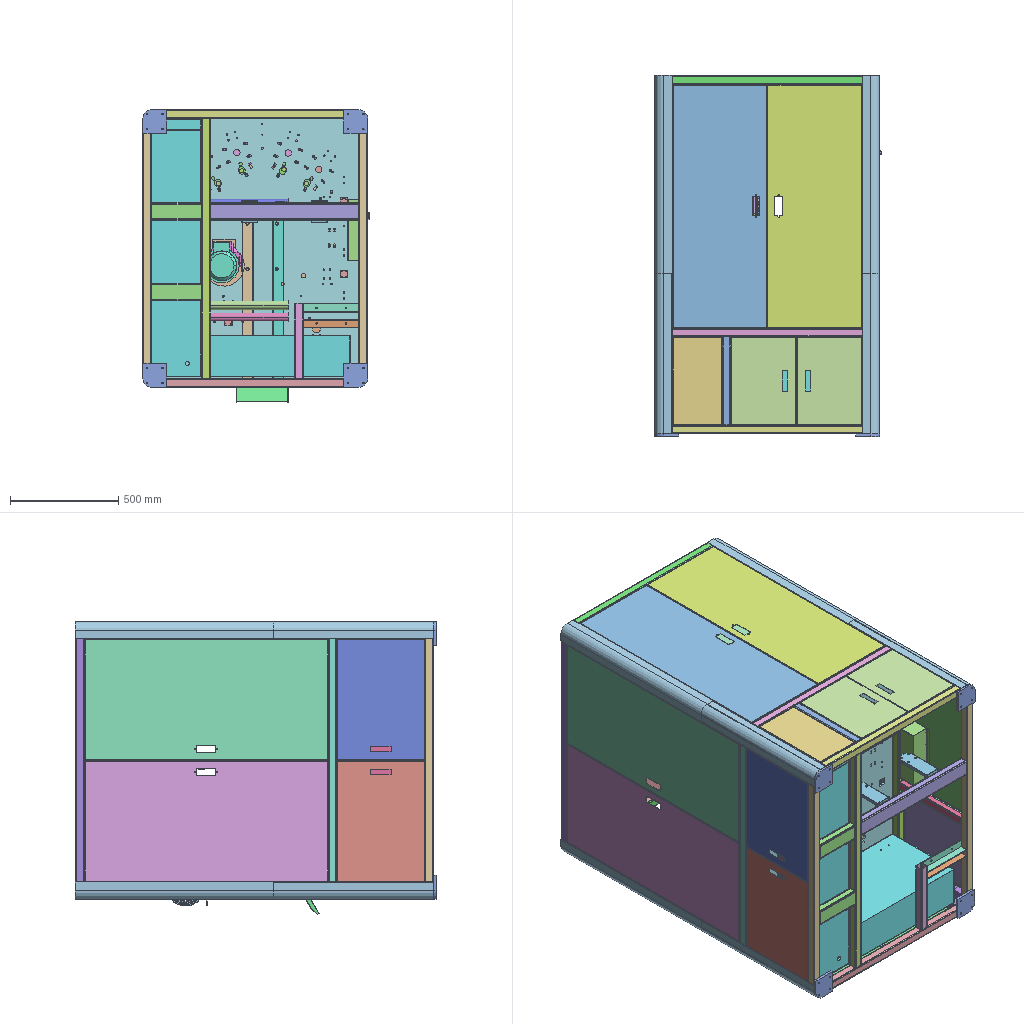Assembly | SolidWorks | 239 different items | 503 placed | box 1043 x 1664 x 1349 mm
Parts list (item | name | quantity | parent item | size | volume):
1 | 1120-1 | x2 | in 26 | - | -
2 | 12X20带轮外购件 | x2 | in 31 | - | -
3 | 4040型材(默认_按加工_) | x1 | in 99 | - | -
4 | 4040角件 | x12 | in 31, 97, 99, 179 | - | -
5 | 4080型材角码 | x17 | in 31, 46, 47, 48, 49, 55, 82 | - | -
6 | 4080型材角码（侧面）  | x4 | in 55 | - | -
7 | 40×40×170型材(默认_按加工_) | x3 | in 82 | - | -
8 | 40×40×220型材(默认_按加工_) | x1 | in 97 | - | -
9 | 40×40×250型材(默认_按加工_) | x1 | in 179 | - | -
10 | 40×80×170型材(默认_按加工_) | x1 | in 82 | - | -
11 | 40×80×400型材-跳火工装6(默认_按加工_) | x1 | in 55 | - | -
12 | 40×80×500型材-跳火工装6(默认_按加工_) | x1 | in 55 | - | -
13 | 40×80×520型材-跳火工装6(默认_按加工_) | x4 | in 46, 47, 48, 49 | - | -
14 | 40×80×560型材-跳火工装6(默认_按加工_) | x2 | in 31 | - | -
15 | 4V210-08-DC24V（单线圈） | x10 | in 31, 55 | - | -
16 | 53-1 | x1 | in 187 | - | -
17 | 80DF+0.55KW普通电机+050减速机(2018-5-28)  2.0  (subassembly) | x1 | in 27 | - | -
18 | 876-1 | x2 | in 26 | - | -
19 | CDM2B20-120Z-XC8B双作用气缸 | x1 | in 31 | - | -
20 | CDM2BZ20x100-D(05) (subassembly) | x1 | in 99 | - | -
21 | CDM2BZ20x120-D(5)_5.stp | x1 | in 20 | 208 x 18 x 18 mm | 11025 mm3
22 | CDM2BZ20x120-D_1.stp | x1 | in 20 | 195 x 24 x 24 mm | 39099 mm3
23 | CDM2BZ20x120-D_2.stp | x1 | in 20 | 7 x 30.022 x 26 mm | 2098 mm3
24 | CDM2BZ20x120-D_3.stp | x1 | in 20 | 6 x 16.166 x 14 mm | 804.447 mm3
25 | CDM2BZ20x170-D(05) (subassembly) | x1 | in 99 | - | -
26 | HL-A-TSJKD-01-MY-MR机架 (subassembly) | x1 | - | - | -
27 | HL-A-TSJKD-02-工作台组件 (subassembly) | x1 | - | - | -
28 | HL-A-TSJKD-02.1-圆盘-工作台1 | x1 | in 27 | - | -
29 | HL-A-TSJKD-02.2-分割器位置检测开光固定架-工作台3 | x1 | in 27 | - | -
30 | HL-A-TSJKD-02.3-1 槽型光电固定钣金(默认) | x1 | in 27 | - | -
31 | HL-A-TSJKD-03-抓取机构 (subassembly) | x1 | - | - | -
32 | HL-A-TSJKD-03.1-1 带轮固定板-抓取机构4(默认_按加工_) | x1 | in 31 | - | -
33 | HL-A-TSJKD-03.1-2 带轮固定板-抓取机构3 | x1 | in 31 | - | -
34 | HL-A-TSJKD-03.2-1.1 12×84的轴-直线模组2 | x1 | in 31 | - | -
35 | HL-A-TSJKD-03.2-1.2 12×65的轴-直线模组-1 | x1 | in 31 | - | -
36 | HL-A-TSJKD-03.3-1 抓取部件1-抓取机构10 | x1 | in 31 | - | -
37 | HL-A-TSJKD-03.3-2 导轨固定架-抓取机构5 | x1 | in 31 | - | -
38 | HL-A-TSJKD-03.3-3 提升卸料支架-跳火传送1 | x1 | in 31 | - | -
39 | HL-A-TSJKD-03.3-4 抓取部件-抓取部件9 | x1 | in 31 | - | -
40 | HL-A-TSJKD-03.3-5 提升卸料板-跳火传送1(默认) | x1 | in 31 | - | -
41 | HL-A-TSJKD-03.5-1 卸料链支架-卸料传动14(默认) | x1 | in 42 | - | -
42 | HL-A-TSJKD-03.5-1 卸料链支架-卸料传动14-成品 (subassembly) | x1 | in 31 | - | -
43 | HL-A-TSJKD-03.5-1 卸料链支架-焊接板 | x1 | in 42 | - | -
44 | HL-A-TSJKD-03.6 压皮带块-抓取机构11 | x2 | in 31 | - | -
45 | HL-A-TSJKD-03.7 感应开关信号架-跳火传送14(默认) | x1 | in 31 | - | -
46 | HL-A-TSJKD-04-跳火工装-1 (subassembly) | x1 | - | - | -
47 | HL-A-TSJKD-04-跳火工装-2 (subassembly) | x1 | - | - | -
48 | HL-A-TSJKD-04-跳火工装-3 (subassembly) | x1 | - | - | -
49 | HL-A-TSJKD-04-跳火工装 (subassembly) | x1 | - | - | -
50 | HL-A-TSJKD-04.1-2 跳火柱支架-跳火传送4 | x8 | in 46, 47, 48, 49 | - | -
51 | HL-A-TSJKD-04.2-1 绝缘托架-跳火工装22 | x4 | in 46, 47, 48, 49 | - | -
52 | HL-A-TSJKD-04.2-2 滑块支座-跳火工装4 | x4 | in 46, 47, 48, 49 | - | -
53 | HL-A-TSJKD-04.3-1 瓷件触电导向-跳火工装16 | x4 | in 46, 47, 48, 49 | - | -
54 | HL-A-TSJKD-04.3-2 抗电针压块-跳火工装5 | x4 | in 46, 47, 48, 49 | - | -
55 | HL-A-TSJKD-05-跳火传送 (subassembly) | x1 | - | - | -
56 | HL-A-TSJKD-05.-6 上料感应开关架-跳火传送1 | x1 | in 55 | - | -
57 | HL-A-TSJKD-05.2-1 传送分料板-跳火传送1 | x1 | in 55 | - | -
58 | HL-A-TSJKD-05.2-2 提升分料组件-跳火传送1 | x1 | in 55 | - | -
59 | HL-A-TSJKD-05.2-3 传送分料坐-跳火传送1 | x1 | in 55 | - | -
60 | HL-A-TSJKD-05.2-4 传送分料板-跳火传送 1 | x2 | in 55 | - | -
61 | HL-A-TSJKD-05.2-5 皮带传送分料板-跳火传送1 | x1 | in 55 | - | -
62 | HL-A-TSJKD-05.2-6 传送分料斗1-跳火传送1 | x4 | in 55 | - | -
63 | HL-A-TSJKD-05.2-7 卸料导向防撞头-跳火传送8 | x4 | in 55 | - | -
64 | HL-A-TSJKD-05.2-8 送料架-跳火传送4 | x4 | in 55 | - | -
65 | HL-A-TSJKD-05.3-1 卸料挡块-跳火直振 | x2 | in 55 | - | -
66 | HL-A-TSJKD-05.3-2 卸料挡块2-跳火直振 | x4 | in 55 | - | -
67 | HL-A-TSJKD-05.4-2 分料气缸接头-跳火传送6 | x1 | in 55 | - | -
68 | HL-A-TSJKD-05.4.1-1 分料气缸架-跳火传送6 | x1 | in 55 | - | -
69 | HL-A-TSJKD-06-卸料传送机构 (subassembly) | x1 | - | - | -
70 | HL-A-TSJKD-06.2-1 卸料槽-卸料传送14-宝玛(默认) | x1 | in 69 | - | -
71 | HL-A-TSJKD-06.2-2 提升卸料槽-跳火传送1(默认) | x1 | in 69 | - | -
72 | HL-A-TSJKD-07-硅胶带传送机构-1 (subassembly) | x1 | - | - | -
73 | HL-A-TSJKD-07-硅胶带传送机构 (subassembly) | x1 | - | - | -
74 | HL-A-TSJKD-07.1-1 硅胶带收轮1-工作台17 | x2 | in 72, 73 | - | -
75 | HL-A-TSJKD-07.1-2 硅胶袋收轮2-工作台17 | x2 | in 72, 73 | - | -
76 | HL-A-TSJKD-07.2-1 硅胶带收料架2-工作台17 | x2 | in 72, 73 | - | -
77 | HL-A-TSJKD-07.2-2 硅胶带收料架1-工作台19-1 | x4 | in 72, 73 | - | -
78 | HL-A-TSJKD-07.2-3 硅胶带传动大架-跳火传送1 | x2 | in 72, 73 | - | -
79 | HL-A-TSJKD-08-气缸顶升机构 (subassembly) | x1 | - | - | -
80 | HL-A-TSJKD-08.1-1 顶升托架-跳火传送 6 | x1 | in 79 | - | -
81 | HL-A-TSJKD-08.1-2 顶升托架-跳火传送6 | x4 | in 79 | - | -
82 | HL-A-TSJKD-09-高压包电柜机构 (subassembly) | x1 | - | - | -
83 | HL-A-TSJKD-09.2-1 电极头-跳火工装14 | x4 | in 82 | - | -
84 | HL-A-TSJKD-09.2-2 电极座-跳火工装5 | x8 | in 82 | - | -
85 | HL-A-TSJKD-09.2-3 80针-跳火工装13 | x8 | in 82 | - | -
86 | HL-A-TSJKD-09.3 三针绝缘板-跳火工装8 | x1 | in 82 | - | -
87 | HL-A-TSJKD-09.3 高压包电柜装配 (subassembly) | x1 | in 82 | - | -
88 | HL-A-TSJKD-09.3-1 包电柜柜体 (subassembly) | x1 | in 87 | - | -
89 | HL-A-TSJKD-09.3-1.1 包电柜柜体 | x1 | in 88 | - | -
90 | HL-A-TSJKD-09.3-1.2 包电柜柜体 | x1 | in 88 | - | -
91 | HL-A-TSJKD-09.3-1.3 包电柜柜体 | x1 | in 88 | - | -
92 | HL-A-TSJKD-09.3-2 包电柜左门 (subassembly) | x1 | in 87 | - | -
93 | HL-A-TSJKD-09.3-2.1 包电柜左门 | x2 | in 92 | - | -
94 | HL-A-TSJKD-09.3-2.2 包电柜左门 | x1 | in 92 | - | -
95 | HL-A-TSJKD-09.3-3 包电柜右门 | x1 | in 87 | - | -
96 | HL-A-TSJKD-09.3-4 高压包电器板(默认SM-FLAT-PATTERN) | x1 | in 82 | - | -
97 | HL-A-TSJKD-10-位置检测机构 (subassembly) | x1 | - | - | -
98 | HL-A-TSJKD-10.1 行程开关固定钣金(默认) | x1 | in 97 | - | -
99 | HL-A-TSJKD-11-抓取机构2 (subassembly) | x1 | - | - | -
100 | HL-A-TSJKD-11.1-1 型材挡块(默认) | x1 | in 99 | - | -
101 | HL-A-TSJKD-11.1-2 气缸安装板(默认) | x1 | in 99 | - | -
102 | HL-A-TSJKD-11.1-3 40×120×300型材(默认_按加工_) | x2 | in 31, 99 | - | -
103 | HL-A-TSJKD-11.1-5 4080-110型材角码 | x1 | in 99 | - | -
104 | HL-A-TSJKD-11.3-1 抓取部件-抓取部件9-2 | x1 | in 99 | - | -
105 | HL-A-TSJKD-11.3-2 抓取部件1-抓取机构10-2 | x1 | in 99 | - | -
106 | HL-A-TSJKD-11.3-3 气缸固定架2-2 | x1 | in 99 | - | -
107 | HL-A-TSJKD-11.3-4 导轨固定架-抓取机构5 | x1 | in 99 | - | -
108 | HL-A-TSJKD-11.3-5 夹头板(默认) | x4 | in 99 | - | -
109 | HL-A-TSJKD-11.3-6 条子(默认) | x4 | in 99 | - | -
110 | HL-A-TSJKD-11.4-1 固定块 | x1 | in 99 | - | -
111 | HL-A-TSJKD-11.4-2 导向块 | x1 | in 99 | - | -
112 | HL-A-TSJKD-11.5-1 卸料链支架-卸料传动14-成品 (subassembly) | x1 | in 99 | - | -
113 | HL-A-TSJKD-11.5-1.1卸料链支架-卸料传动14(默认) | x1 | in 112 | - | -
114 | HL-A-TSJKD-11.5-1.2卸料链支架-焊接板 | x1 | in 112 | - | -
115 | HL-A-TSJKD-12-电磁阀安装板-跳火工装10 | x1 | - | - | -
116 | HL-A-TSJKD-13-硅胶盘支架-卸料传送14-宝玛(默认) | x2 | - | - | -
117 | HL-A-TSJKD-14-承座限位板(默认) | x1 | - | - | -
118 | HL-A-TSJKD-15-料盒安装板(默认) | x1 | - | - | -
119 | HL-A-TSJKD-16-废品盒固定块(默认) | x1 | - | - | -
120 | HL-A-TSJKD-光敏盒压条(默认) | x1 | in 26 | - | -
121 | HL-A-TSJKD-大板202664 | x1 | in 26 | - | -
122 | HL-A-TSJKD-电器板(默认) | x1 | in 187 | - | -
123 | MHZ2-20D-M9BW气缸 卸料-外购件(1) | x2 | in 99 | - | -
124 | S-SDA25x35-S-B(0_0).stp (subassembly) | x1 | in 55 | 89 x 40 x 42 mm | 65773 mm3
125 | S-SDA25x35-SB(0)_rod.stp | x1 | in 124 | 84 x 16.166 x 14.001 mm | 6760 mm3
126 | S-SDA25x35-SB_body.stp | x1 | in 124 | 68 x 40 x 42 mm | 59012 mm3
127 | TL-Q5MC1-Z电感式传感器(OMRON) | x2 | in 31 | - | -
128 | TRH15A直线导轨15×15×185.SLDPRT | x2 | in 31, 99 | - | -
129 | TRH15A直线导轨15×15×205 | x8 | in 46, 47, 48, 49 | - | -
130 | TRH15A直线导轨15×15×236 | x1 | in 55 | - | -
131 | TRH15A直线导轨15×15×298 | x4 | in 31, 99 | - | -
132 | YBLX-ME_8169行程开关 | x1 | in 97 | - | -
133 | 下机架框架-002-2_1_1DrPart-002-1-1 | x4 | in 187 | - | -
134 | 下机架框架-008-2_1_1DrPart-008-1-1 | x1 | in 187 | - | -
135 | 下机架框架-009-2_1_1DrPart-009-1-1 | x1 | in 187 | - | -
136 | 下机架框架-012-2_1_1DrPart-012-1-1 | x1 | in 187 | - | -
137 | 下机架框架-015-2_1_1DrPart-015-1-1 | x1 | in 187 | - | -
138 | 伺服电机联轴器外径30长度42 孔12-14-外购件 | x1 | in 31 | - | -
139 | 台达伺服电机ECMA -CX0604ES | x1 | in 31 | - | -
140 | 同步带 | x1 | in 31 | - | -
141 | 圆角堵头-1-1 | x1 | in 26 | - | -
142 | 型材框架-2-1-1-1 (subassembly) | x1 | in 26 | - | -
143 | 型材端盖ARC52-4010-H4040 | x2 | in 97, 179 | - | -
144 | 复件 CDM2BZ20x180-D(5)_5^CDM2BZ20x170-D(05) | x1 | in 25 | - | -
145 | 复件 CDM2BZ20x180-D_1^CDM2BZ20x170-D(05) | x1 | in 25 | - | -
146 | 复件 CDM2BZ20x180-D_2^CDM2BZ20x170-D(05) | x1 | in 25 | - | -
147 | 复件 CDM2BZ20x180-D_3^CDM2BZ20x170-D(05) | x1 | in 25 | - | -
148 | 复件 MGPL-63x25_body1^气缸MGPL-63x25 | x2 | in 194, 195 | - | -
149 | 复件 MGPL-63x25_body2^气缸MGPL-63x25 | x2 | in 194, 195 | - | -
150 | - | x1 | in 196 | - | -
151 | - | x1 | in 196 | - | -
152 | - | x1 | in 196 | - | -
153 | - | x1 | in 196 | - | -
154 | - | x1 | in 196 | - | -
155 | - | x2 | in 196 | - | -
156 | - | x1 | in 196 | - | -
157 | - | x2 | in 196 | - | -
158 | 复件 _CS1-E()-1^标准气缸SE32x80S_000_+_CMSE-2_ | x8 | in 190, 191, 192, 193 | - | -
159 | 复件 _SE-32-M10x1.25 - Nut^标准气缸DNC32x80S_000_+_CMSE-2_ | x4 | in 190, 191, 192, 193 | - | -
160 | 复件 _SE-3280_SE^标准气缸DNC32x80S_000_+_CMSE-2_ | x4 | in 190, 191, 192, 193 | - | -
161 | 复件 _SE-32x80-S(0)_r^标准气缸DNC32x80S_000_+_CMSE-2_ | x4 | in 190, 191, 192, 193 | - | -
162 | 复件 _VBD32-F25-R75-N17-001^拖链VBD32-F25-R75-N17 | x34 | in 184, 185 | - | -
163 | 复件 _VED32-F25-001^拖链VBD32-F25-R75-N17 | x2 | in 184, 185 | - | -
164 | 复件 _VED32-F25-002^拖链VBD32-F25-R75-N17 | x2 | in 184, 185 | - | -
165 | - | x3 | in 197, 198, 199 | - | -
166 | - | x4 | in 200, 201, 202, 203 | - | -
167 | - | x3 | in 197, 198, 199 | - | -
168 | - | x4 | in 200, 201, 202, 203 | - | -
169 | - | x2 | in 196 | - | -
170 | - | x1 | in 196 | - | -
171 | - | x3 | in 197, 198, 199 | - | -
172 | - | x4 | in 200, 201, 202, 203 | - | -
173 | - | x3 | in 197, 198, 199 | - | -
174 | - | x4 | in 200, 201, 202, 203 | - | -
175 | 复件 实体1 | x1 | in 17 | - | -
176 | 复件 实体2 | x1 | in 17 | - | -
177 | 复件 实体3 | x1 | in 17 | - | -
178 | 复件 实体4 | x1 | in 17 | - | -
179 | 安装型材 (subassembly) | x1 | in 69 | - | -
180 | 宝华电机-BF37GB24-60  DC24v 60RMP | x2 | in 72, 73 | - | -
181 | 封板-1-1 | x1 | in 187 | - | -
182 | 封板_1(默认)-1-1 | x1 | in 142 | - | -
183 | 悬臂控制箱 | x1 | - | - | -
184 | 拖链VBD32-F25-R75-N17-1 (subassembly) | x1 | in 99 | - | -
185 | 拖链VBD32-F25-R75-N17 (subassembly) | x1 | in 31 | - | -
186 | 方管-1-1 | x1 | in 187 | - | -
187 | 板条下机架-2-1-1-1 (subassembly) | x1 | in 26 | - | -
188 | 框架DrPart-1-1 | x1 | in 187 | - | -
189 | 槽型光电 | x1 | in 27 | - | -
190 | 气缸DNC32x80-PPV-A(0_0)-1 (subassembly) | x1 | in 46 | - | -
191 | 气缸DNC32x80-PPV-A(0_0)-2 (subassembly) | x1 | in 47 | - | -
192 | 气缸DNC32x80-PPV-A(0_0)-3 (subassembly) | x1 | in 48 | - | -
193 | 气缸DNC32x80-PPV-A(0_0) (subassembly) | x1 | in 49 | - | -
194 | 气缸MGPL-63x25-1 (subassembly) | x1 | in 72 | - | -
195 | 气缸MGPL-63x25 (subassembly) | x1 | in 73 | - | -
196 | 气缸MGPM20x30 (subassembly) | x1 | in 79 | - | -
197 | 浮动接头FJ-1008M8X1.25-1 (subassembly) | x1 | in 55 | - | -
198 | 浮动接头FJ-1008M8X1.25-2 (subassembly) | x1 | in 99 | - | -
199 | 浮动接头FJ-1008M8X1.25 (subassembly) | x1 | in 31 | - | -
200 | 浮动接头FJ-1010M10X1.25-1 (subassembly) | x1 | in 46 | - | -
201 | 浮动接头FJ-1010M10X1.25-2 (subassembly) | x1 | in 47 | - | -
202 | 浮动接头FJ-1010M10X1.25-3 (subassembly) | x1 | in 48 | - | -
203 | 浮动接头FJ-1010M10X1.25 (subassembly) | x1 | in 49 | - | -
204 | 滑块-外购件（TRH15A直线导轨块） | x16 | in 31, 46, 47, 48, 49, 55, 99 | - | -
205 | 焊接螺柱 | x4 | in 82 | - | -
206 | 硅胶管 | x1 | in 31 | - | -
207 | 立式KP001轴承套-外购件 | x4 | in 31 | - | -
208 | 绝缘子 | x4 | in 46, 47, 48, 49 | - | -
209 | 螺柱 焊 | x2 | in 26 | - | -
210 | 螺柱 | x4 | in 46, 47, 48, 49 | - | -
211 | 角码-3 | x2 | in 26 | - | -
212 | 轴承 外径11内径5厚度5 | x4 | in 72, 73 | - | -
213 | 迷你-u夹爪 | x4 | in 31 | - | -
214 | 钣金2镜像-1 | x1 | in 26 | - | -
215 | 钣金罩 | x1 | in 26 | - | -
216 | 钣金门-1-1 | x1 | in 187 | - | -
217 | 钣金门1-3 | x1 | in 26 | - | -
218 | 钣金门2-3 | x1 | in 26 | - | -
219 | 门板-1-1-1-1 | x1 | in 26 | - | -
220 | 门板-2-1-1-1 | x1 | in 26 | - | -
221 | 门板-3-1-1 | x2 | in 26 | - | -
222 | 零件1镜像-1 | x1 | in 26 | - | -
223 | 零件26-1 | x1 | in 26 | - | -
224 | 零件28-1 | x4 | in 187 | - | -
225 | 零件48-1-1 | x1 | in 187 | - | -
226 | 零件50-1-1 | x8 | in 187 | - | -
227 | 零件51-1-1 | x2 | in 187 | - | -
228 | 零件52-1 | x3 | in 187 | - | -
229 | 零件53-1 | x2 | in 26 | - | -
230 | 零件54-1-1 | x2 | in 26, 187 | - | -
231 | 零件55-1-1 | x1 | in 187 | - | -
232 | 零件56-1-1 | x1 | in 187 | - | -
233 | 零件57(默认_按加工_)-1 | x1 | in 187 | - | -
234 | 零件58(默认_按加工_)-1 | x1 | in 187 | - | -
235 | 零件59(默认_按加工_)-1 | x2 | in 187 | - | -
236 | 零件60(默认_按加工_)-1 | x1 | in 26 | - | -
237 | 零件62-1-1.1-2 | x1 | in 26 | - | -
238 | 零件62-1-1 | x1 | in 26 | - | -
239 | 零件8 | x1 | in 26 | - | -